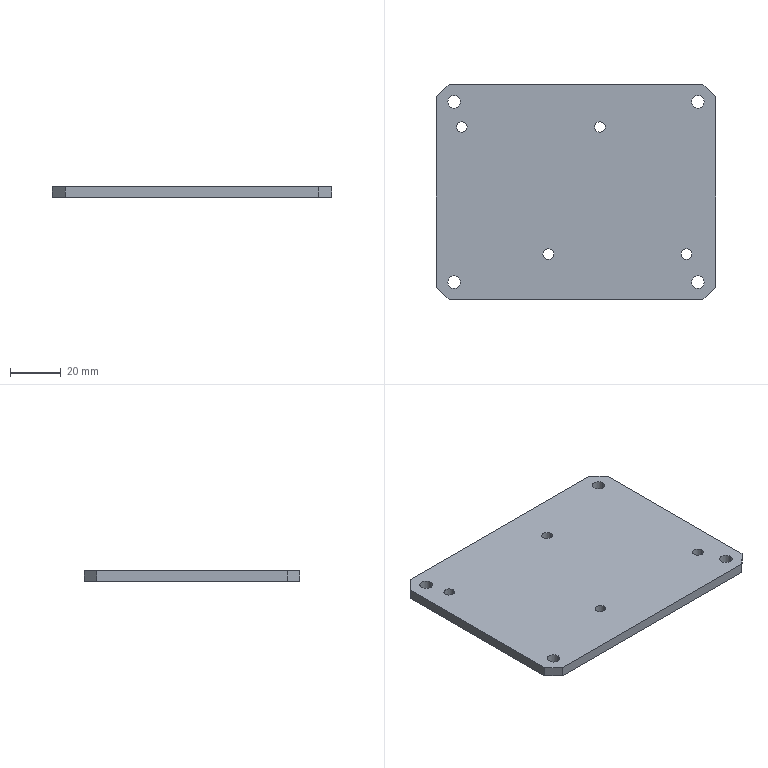Part | SolidWorks | features HoleWzd 2, Chamfer 1, Extrusion 1 | 1 solid | 26 faces | box 110 x 85 x 4 mm | volume 36664 mm3 | cylinder 16 | plane 10 | commonest cylinder face diameters 4.2 x8 5 x8
STEP:
#1=CARTESIAN_POINT('',(-71.534,24.385,4.));
#2=VERTEX_POINT('',#1);
#3=CARTESIAN_POINT('',(-66.534,24.385,4.));
#4=VERTEX_POINT('',#3);
#5=CARTESIAN_POINT('',(-69.034,24.385,4.));
#6=DIRECTION('',(0.,0.,1.));
#7=DIRECTION('',(1.,0.,0.));
#8=AXIS2_PLACEMENT_3D('',#5,#6,#7);
#9=CIRCLE('',#8,2.5);
#10=EDGE_CURVE('',#2,#4,#9,.T.);
#11=ORIENTED_EDGE('',*,*,#10,.T.);
#12=CARTESIAN_POINT('',(-66.534,24.385,0.));
#13=VERTEX_POINT('',#12);
#14=CARTESIAN_POINT('',(-66.534,24.385,0.));
#15=DIRECTION('',(0.,0.,-1.));
#16=VECTOR('',#15,1000.);
#17=LINE('',#14,#16);
#18=EDGE_CURVE('',#4,#13,#17,.T.);
#19=ORIENTED_EDGE('',*,*,#18,.T.);
#20=CARTESIAN_POINT('',(-71.534,24.385,0.));
#21=VERTEX_POINT('',#20);
#22=CARTESIAN_POINT('',(-69.034,24.385,0.));
#23=DIRECTION('',(0.,0.,-1.));
#24=DIRECTION('',(-1.,0.,0.));
#25=AXIS2_PLACEMENT_3D('',#22,#23,#24);
#26=CIRCLE('',#25,2.5);
#27=EDGE_CURVE('',#13,#21,#26,.T.);
#28=ORIENTED_EDGE('',*,*,#27,.T.);
#29=CARTESIAN_POINT('',(-71.534,24.385,0.));
#30=DIRECTION('',(0.,0.,-1.));
#31=VECTOR('',#30,1000.);
#32=LINE('',#29,#31);
#33=EDGE_CURVE('',#2,#21,#32,.T.);
#34=ORIENTED_EDGE('',*,*,#33,.F.);
#35=EDGE_LOOP('',(#11,#19,#28,#34));
#36=FACE_OUTER_BOUND('',#35,.T.);
#37=CARTESIAN_POINT('',(-69.034,24.385,0.));
#38=DIRECTION('',(0.,0.,-1.));
#39=DIRECTION('',(-1.,0.,0.));
#40=AXIS2_PLACEMENT_3D('',#37,#38,#39);
#41=CYLINDRICAL_SURFACE('',#40,2.5);
#42=ADVANCED_FACE('',(#36),#41,.F.);
#43=CARTESIAN_POINT('',(-71.534,-46.615,4.));
#44=VERTEX_POINT('',#43);
#45=CARTESIAN_POINT('',(-66.534,-46.615,4.));
#46=VERTEX_POINT('',#45);
#47=CARTESIAN_POINT('',(-69.034,-46.615,4.));
#48=DIRECTION('',(0.,0.,1.));
#49=DIRECTION('',(1.,0.,0.));
#50=AXIS2_PLACEMENT_3D('',#47,#48,#49);
#51=CIRCLE('',#50,2.5);
#52=EDGE_CURVE('',#44,#46,#51,.T.);
#53=ORIENTED_EDGE('',*,*,#52,.T.);
#54=CARTESIAN_POINT('',(-66.534,-46.615,0.));
#55=VERTEX_POINT('',#54);
#56=CARTESIAN_POINT('',(-66.534,-46.615,0.));
#57=DIRECTION('',(0.,0.,-1.));
#58=VECTOR('',#57,1000.);
#59=LINE('',#56,#58);
#60=EDGE_CURVE('',#46,#55,#59,.T.);
#61=ORIENTED_EDGE('',*,*,#60,.T.);
#62=CARTESIAN_POINT('',(-71.534,-46.615,0.));
#63=VERTEX_POINT('',#62);
#64=CARTESIAN_POINT('',(-69.034,-46.615,0.));
#65=DIRECTION('',(0.,0.,-1.));
#66=DIRECTION('',(-1.,0.,0.));
#67=AXIS2_PLACEMENT_3D('',#64,#65,#66);
#68=CIRCLE('',#67,2.5);
#69=EDGE_CURVE('',#55,#63,#68,.T.);
#70=ORIENTED_EDGE('',*,*,#69,.T.);
#71=CARTESIAN_POINT('',(-71.534,-46.615,0.));
#72=DIRECTION('',(0.,0.,-1.));
#73=VECTOR('',#72,1000.);
#74=LINE('',#71,#73);
#75=EDGE_CURVE('',#44,#63,#74,.T.);
#76=ORIENTED_EDGE('',*,*,#75,.F.);
#77=EDGE_LOOP('',(#53,#61,#70,#76));
#78=FACE_OUTER_BOUND('',#77,.T.);
#79=CARTESIAN_POINT('',(-69.034,-46.615,0.));
#80=DIRECTION('',(0.,0.,-1.));
#81=DIRECTION('',(-1.,0.,0.));
#82=AXIS2_PLACEMENT_3D('',#79,#80,#81);
#83=CYLINDRICAL_SURFACE('',#82,2.5);
#84=ADVANCED_FACE('',(#78),#83,.F.);
#85=CARTESIAN_POINT('',(24.466,-46.615,4.));
#86=VERTEX_POINT('',#85);
#87=CARTESIAN_POINT('',(29.466,-46.615,4.));
#88=VERTEX_POINT('',#87);
#89=CARTESIAN_POINT('',(26.966,-46.615,4.));
#90=DIRECTION('',(0.,0.,1.));
#91=DIRECTION('',(1.,0.,0.));
#92=AXIS2_PLACEMENT_3D('',#89,#90,#91);
#93=CIRCLE('',#92,2.5);
#94=EDGE_CURVE('',#86,#88,#93,.T.);
#95=ORIENTED_EDGE('',*,*,#94,.T.);
#96=CARTESIAN_POINT('',(29.466,-46.615,0.));
#97=VERTEX_POINT('',#96);
#98=CARTESIAN_POINT('',(29.466,-46.615,0.));
#99=DIRECTION('',(0.,0.,-1.));
#100=VECTOR('',#99,1000.);
#101=LINE('',#98,#100);
#102=EDGE_CURVE('',#88,#97,#101,.T.);
#103=ORIENTED_EDGE('',*,*,#102,.T.);
#104=CARTESIAN_POINT('',(24.466,-46.615,0.));
#105=VERTEX_POINT('',#104);
#106=CARTESIAN_POINT('',(26.966,-46.615,0.));
#107=DIRECTION('',(0.,0.,-1.));
#108=DIRECTION('',(-1.,0.,0.));
#109=AXIS2_PLACEMENT_3D('',#106,#107,#108);
#110=CIRCLE('',#109,2.5);
#111=EDGE_CURVE('',#97,#105,#110,.T.);
#112=ORIENTED_EDGE('',*,*,#111,.T.);
#113=CARTESIAN_POINT('',(24.466,-46.615,0.));
#114=DIRECTION('',(0.,0.,-1.));
#115=VECTOR('',#114,1000.);
#116=LINE('',#113,#115);
#117=EDGE_CURVE('',#86,#105,#116,.T.);
#118=ORIENTED_EDGE('',*,*,#117,.F.);
#119=EDGE_LOOP('',(#95,#103,#112,#118));
#120=FACE_OUTER_BOUND('',#119,.T.);
#121=CARTESIAN_POINT('',(26.966,-46.615,0.));
#122=DIRECTION('',(0.,0.,-1.));
#123=DIRECTION('',(-1.,0.,0.));
#124=AXIS2_PLACEMENT_3D('',#121,#122,#123);
#125=CYLINDRICAL_SURFACE('',#124,2.5);
#126=ADVANCED_FACE('',(#120),#125,.F.);
#127=CARTESIAN_POINT('',(24.466,24.385,4.));
#128=VERTEX_POINT('',#127);
#129=CARTESIAN_POINT('',(29.466,24.385,4.));
#130=VERTEX_POINT('',#129);
#131=CARTESIAN_POINT('',(26.966,24.385,4.));
#132=DIRECTION('',(0.,0.,1.));
#133=DIRECTION('',(1.,0.,0.));
#134=AXIS2_PLACEMENT_3D('',#131,#132,#133);
#135=CIRCLE('',#134,2.5);
#136=EDGE_CURVE('',#128,#130,#135,.T.);
#137=ORIENTED_EDGE('',*,*,#136,.T.);
#138=CARTESIAN_POINT('',(29.466,24.385,0.));
#139=VERTEX_POINT('',#138);
#140=CARTESIAN_POINT('',(29.466,24.385,0.));
#141=DIRECTION('',(0.,0.,-1.));
#142=VECTOR('',#141,1000.);
#143=LINE('',#140,#142);
#144=EDGE_CURVE('',#130,#139,#143,.T.);
#145=ORIENTED_EDGE('',*,*,#144,.T.);
#146=CARTESIAN_POINT('',(24.466,24.385,0.));
#147=VERTEX_POINT('',#146);
#148=CARTESIAN_POINT('',(26.966,24.385,0.));
#149=DIRECTION('',(0.,0.,-1.));
#150=DIRECTION('',(-1.,0.,0.));
#151=AXIS2_PLACEMENT_3D('',#148,#149,#150);
#152=CIRCLE('',#151,2.5);
#153=EDGE_CURVE('',#139,#147,#152,.T.);
#154=ORIENTED_EDGE('',*,*,#153,.T.);
#155=CARTESIAN_POINT('',(24.466,24.385,0.));
#156=DIRECTION('',(0.,0.,-1.));
#157=VECTOR('',#156,1000.);
#158=LINE('',#155,#157);
#159=EDGE_CURVE('',#128,#147,#158,.T.);
#160=ORIENTED_EDGE('',*,*,#159,.F.);
#161=EDGE_LOOP('',(#137,#145,#154,#160));
#162=FACE_OUTER_BOUND('',#161,.T.);
#163=CARTESIAN_POINT('',(26.966,24.385,0.));
#164=DIRECTION('',(0.,0.,-1.));
#165=DIRECTION('',(-1.,0.,0.));
#166=AXIS2_PLACEMENT_3D('',#163,#164,#165);
#167=CYLINDRICAL_SURFACE('',#166,2.5);
#168=ADVANCED_FACE('',(#162),#167,.F.);
#169=CARTESIAN_POINT('',(-68.134,14.495,0.));
#170=VERTEX_POINT('',#169);
#171=CARTESIAN_POINT('',(-63.934,14.495,0.));
#172=VERTEX_POINT('',#171);
#173=CARTESIAN_POINT('',(-66.034,14.495,0.));
#174=DIRECTION('',(0.,0.,1.));
#175=DIRECTION('',(1.,0.,0.));
#176=AXIS2_PLACEMENT_3D('',#173,#174,#175);
#177=CIRCLE('',#176,2.1);
#178=EDGE_CURVE('',#170,#172,#177,.T.);
#179=ORIENTED_EDGE('',*,*,#178,.F.);
#180=CARTESIAN_POINT('',(-68.134,14.495,4.));
#181=VERTEX_POINT('',#180);
#182=CARTESIAN_POINT('',(-68.134,14.495,4.));
#183=DIRECTION('',(0.,0.,1.));
#184=VECTOR('',#183,1000.);
#185=LINE('',#182,#184);
#186=EDGE_CURVE('',#170,#181,#185,.T.);
#187=ORIENTED_EDGE('',*,*,#186,.T.);
#188=CARTESIAN_POINT('',(-63.934,14.495,4.));
#189=VERTEX_POINT('',#188);
#190=CARTESIAN_POINT('',(-66.034,14.495,4.));
#191=DIRECTION('',(0.,0.,1.));
#192=DIRECTION('',(1.,0.,0.));
#193=AXIS2_PLACEMENT_3D('',#190,#191,#192);
#194=CIRCLE('',#193,2.1);
#195=EDGE_CURVE('',#181,#189,#194,.T.);
#196=ORIENTED_EDGE('',*,*,#195,.T.);
#197=CARTESIAN_POINT('',(-63.934,14.495,4.));
#198=DIRECTION('',(0.,0.,1.));
#199=VECTOR('',#198,1000.);
#200=LINE('',#197,#199);
#201=EDGE_CURVE('',#172,#189,#200,.T.);
#202=ORIENTED_EDGE('',*,*,#201,.F.);
#203=EDGE_LOOP('',(#179,#187,#196,#202));
#204=FACE_OUTER_BOUND('',#203,.T.);
#205=CARTESIAN_POINT('',(-66.034,14.495,4.));
#206=DIRECTION('',(0.,0.,1.));
#207=DIRECTION('',(1.,0.,0.));
#208=AXIS2_PLACEMENT_3D('',#205,#206,#207);
#209=CYLINDRICAL_SURFACE('',#208,2.1);
#210=ADVANCED_FACE('',(#204),#209,.F.);
#211=CARTESIAN_POINT('',(-34.054,-35.615,0.));
#212=VERTEX_POINT('',#211);
#213=CARTESIAN_POINT('',(-29.854,-35.615,0.));
#214=VERTEX_POINT('',#213);
#215=CARTESIAN_POINT('',(-31.954,-35.615,0.));
#216=DIRECTION('',(0.,0.,1.));
#217=DIRECTION('',(1.,0.,0.));
#218=AXIS2_PLACEMENT_3D('',#215,#216,#217);
#219=CIRCLE('',#218,2.1);
#220=EDGE_CURVE('',#212,#214,#219,.T.);
#221=ORIENTED_EDGE('',*,*,#220,.F.);
#222=CARTESIAN_POINT('',(-34.054,-35.615,4.));
#223=VERTEX_POINT('',#222);
#224=CARTESIAN_POINT('',(-34.054,-35.615,4.));
#225=DIRECTION('',(0.,0.,1.));
#226=VECTOR('',#225,1000.);
#227=LINE('',#224,#226);
#228=EDGE_CURVE('',#212,#223,#227,.T.);
#229=ORIENTED_EDGE('',*,*,#228,.T.);
#230=CARTESIAN_POINT('',(-29.854,-35.615,4.));
#231=VERTEX_POINT('',#230);
#232=CARTESIAN_POINT('',(-31.954,-35.615,4.));
#233=DIRECTION('',(0.,0.,1.));
#234=DIRECTION('',(1.,0.,0.));
#235=AXIS2_PLACEMENT_3D('',#232,#233,#234);
#236=CIRCLE('',#235,2.1);
#237=EDGE_CURVE('',#223,#231,#236,.T.);
#238=ORIENTED_EDGE('',*,*,#237,.T.);
#239=CARTESIAN_POINT('',(-29.854,-35.615,4.));
#240=DIRECTION('',(0.,0.,1.));
#241=VECTOR('',#240,1000.);
#242=LINE('',#239,#241);
#243=EDGE_CURVE('',#214,#231,#242,.T.);
#244=ORIENTED_EDGE('',*,*,#243,.F.);
#245=EDGE_LOOP('',(#221,#229,#238,#244));
#246=FACE_OUTER_BOUND('',#245,.T.);
#247=CARTESIAN_POINT('',(-31.954,-35.615,4.));
#248=DIRECTION('',(0.,0.,1.));
#249=DIRECTION('',(1.,0.,0.));
#250=AXIS2_PLACEMENT_3D('',#247,#248,#249);
#251=CYLINDRICAL_SURFACE('',#250,2.1);
#252=ADVANCED_FACE('',(#246),#251,.F.);
#253=CARTESIAN_POINT('',(-13.714,14.495,0.));
#254=VERTEX_POINT('',#253);
#255=CARTESIAN_POINT('',(-9.514,14.495,0.));
#256=VERTEX_POINT('',#255);
#257=CARTESIAN_POINT('',(-11.614,14.495,0.));
#258=DIRECTION('',(0.,0.,1.));
#259=DIRECTION('',(1.,0.,0.));
#260=AXIS2_PLACEMENT_3D('',#257,#258,#259);
#261=CIRCLE('',#260,2.1);
#262=EDGE_CURVE('',#254,#256,#261,.T.);
#263=ORIENTED_EDGE('',*,*,#262,.F.);
#264=CARTESIAN_POINT('',(-13.714,14.495,4.));
#265=VERTEX_POINT('',#264);
#266=CARTESIAN_POINT('',(-13.714,14.495,4.));
#267=DIRECTION('',(0.,0.,1.));
#268=VECTOR('',#267,1000.);
#269=LINE('',#266,#268);
#270=EDGE_CURVE('',#254,#265,#269,.T.);
#271=ORIENTED_EDGE('',*,*,#270,.T.);
#272=CARTESIAN_POINT('',(-9.514,14.495,4.));
#273=VERTEX_POINT('',#272);
#274=CARTESIAN_POINT('',(-11.614,14.495,4.));
#275=DIRECTION('',(0.,0.,1.));
#276=DIRECTION('',(1.,0.,0.));
#277=AXIS2_PLACEMENT_3D('',#274,#275,#276);
#278=CIRCLE('',#277,2.1);
#279=EDGE_CURVE('',#265,#273,#278,.T.);
#280=ORIENTED_EDGE('',*,*,#279,.T.);
#281=CARTESIAN_POINT('',(-9.514,14.495,4.));
#282=DIRECTION('',(0.,0.,1.));
#283=VECTOR('',#282,1000.);
#284=LINE('',#281,#283);
#285=EDGE_CURVE('',#256,#273,#284,.T.);
#286=ORIENTED_EDGE('',*,*,#285,.F.);
#287=EDGE_LOOP('',(#263,#271,#280,#286));
#288=FACE_OUTER_BOUND('',#287,.T.);
#289=CARTESIAN_POINT('',(-11.614,14.495,4.));
#290=DIRECTION('',(0.,0.,1.));
#291=DIRECTION('',(1.,0.,0.));
#292=AXIS2_PLACEMENT_3D('',#289,#290,#291);
#293=CYLINDRICAL_SURFACE('',#292,2.1);
#294=ADVANCED_FACE('',(#288),#293,.F.);
#295=CARTESIAN_POINT('',(20.366,-35.615,0.));
#296=VERTEX_POINT('',#295);
#297=CARTESIAN_POINT('',(24.566,-35.615,0.));
#298=VERTEX_POINT('',#297);
#299=CARTESIAN_POINT('',(22.466,-35.615,0.));
#300=DIRECTION('',(0.,0.,1.));
#301=DIRECTION('',(1.,0.,0.));
#302=AXIS2_PLACEMENT_3D('',#299,#300,#301);
#303=CIRCLE('',#302,2.1);
#304=EDGE_CURVE('',#296,#298,#303,.T.);
#305=ORIENTED_EDGE('',*,*,#304,.F.);
#306=CARTESIAN_POINT('',(20.366,-35.615,4.));
#307=VERTEX_POINT('',#306);
#308=CARTESIAN_POINT('',(20.366,-35.615,4.));
#309=DIRECTION('',(0.,0.,1.));
#310=VECTOR('',#309,1000.);
#311=LINE('',#308,#310);
#312=EDGE_CURVE('',#296,#307,#311,.T.);
#313=ORIENTED_EDGE('',*,*,#312,.T.);
#314=CARTESIAN_POINT('',(24.566,-35.615,4.));
#315=VERTEX_POINT('',#314);
#316=CARTESIAN_POINT('',(22.466,-35.615,4.));
#317=DIRECTION('',(0.,0.,1.));
#318=DIRECTION('',(1.,0.,0.));
#319=AXIS2_PLACEMENT_3D('',#316,#317,#318);
#320=CIRCLE('',#319,2.1);
#321=EDGE_CURVE('',#307,#315,#320,.T.);
#322=ORIENTED_EDGE('',*,*,#321,.T.);
#323=CARTESIAN_POINT('',(24.566,-35.615,4.));
#324=DIRECTION('',(0.,0.,1.));
#325=VECTOR('',#324,1000.);
#326=LINE('',#323,#325);
#327=EDGE_CURVE('',#298,#315,#326,.T.);
#328=ORIENTED_EDGE('',*,*,#327,.F.);
#329=EDGE_LOOP('',(#305,#313,#322,#328));
#330=FACE_OUTER_BOUND('',#329,.T.);
#331=CARTESIAN_POINT('',(22.466,-35.615,4.));
#332=DIRECTION('',(0.,0.,1.));
#333=DIRECTION('',(1.,0.,0.));
#334=AXIS2_PLACEMENT_3D('',#331,#332,#333);
#335=CYLINDRICAL_SURFACE('',#334,2.1);
#336=ADVANCED_FACE('',(#330),#335,.F.);
#337=CARTESIAN_POINT('',(-69.034,24.385,0.));
#338=DIRECTION('',(0.,0.,-1.));
#339=DIRECTION('',(-1.,0.,0.));
#340=AXIS2_PLACEMENT_3D('',#337,#338,#339);
#341=CIRCLE('',#340,2.5);
#342=EDGE_CURVE('',#21,#13,#341,.T.);
#343=ORIENTED_EDGE('',*,*,#342,.F.);
#344=ORIENTED_EDGE('',*,*,#27,.F.);
#345=EDGE_LOOP('',(#343,#344));
#346=FACE_BOUND('',#345,.T.);
#347=CARTESIAN_POINT('',(-69.034,-46.615,0.));
#348=DIRECTION('',(0.,0.,-1.));
#349=DIRECTION('',(-1.,0.,0.));
#350=AXIS2_PLACEMENT_3D('',#347,#348,#349);
#351=CIRCLE('',#350,2.5);
#352=EDGE_CURVE('',#63,#55,#351,.T.);
#353=ORIENTED_EDGE('',*,*,#352,.F.);
#354=ORIENTED_EDGE('',*,*,#69,.F.);
#355=EDGE_LOOP('',(#353,#354));
#356=FACE_BOUND('',#355,.T.);
#357=CARTESIAN_POINT('',(26.966,-46.615,0.));
#358=DIRECTION('',(0.,0.,-1.));
#359=DIRECTION('',(-1.,0.,0.));
#360=AXIS2_PLACEMENT_3D('',#357,#358,#359);
#361=CIRCLE('',#360,2.5);
#362=EDGE_CURVE('',#105,#97,#361,.T.);
#363=ORIENTED_EDGE('',*,*,#362,.F.);
#364=ORIENTED_EDGE('',*,*,#111,.F.);
#365=EDGE_LOOP('',(#363,#364));
#366=FACE_BOUND('',#365,.T.);
#367=CARTESIAN_POINT('',(-71.034,-53.615,0.));
#368=VERTEX_POINT('',#367);
#369=CARTESIAN_POINT('',(28.966,-53.615,0.));
#370=VERTEX_POINT('',#369);
#371=CARTESIAN_POINT('',(-76.034,-53.615,0.));
#372=DIRECTION('',(1.,0.,0.));
#373=VECTOR('',#372,1000.);
#374=LINE('',#371,#373);
#375=EDGE_CURVE('',#368,#370,#374,.T.);
#376=ORIENTED_EDGE('',*,*,#375,.F.);
#377=CARTESIAN_POINT('',(-76.034,-48.615,0.));
#378=VERTEX_POINT('',#377);
#379=CARTESIAN_POINT('',(-71.034,-53.615,0.));
#380=DIRECTION('',(-0.7071,0.7071,0.));
#381=VECTOR('',#380,1000.);
#382=LINE('',#379,#381);
#383=EDGE_CURVE('',#368,#378,#382,.T.);
#384=ORIENTED_EDGE('',*,*,#383,.T.);
#385=CARTESIAN_POINT('',(-76.034,26.385,0.));
#386=VERTEX_POINT('',#385);
#387=CARTESIAN_POINT('',(-76.034,31.385,0.));
#388=DIRECTION('',(0.,-1.,0.));
#389=VECTOR('',#388,1000.);
#390=LINE('',#387,#389);
#391=EDGE_CURVE('',#386,#378,#390,.T.);
#392=ORIENTED_EDGE('',*,*,#391,.F.);
#393=CARTESIAN_POINT('',(-71.034,31.385,0.));
#394=VERTEX_POINT('',#393);
#395=CARTESIAN_POINT('',(-76.034,26.385,0.));
#396=DIRECTION('',(0.7071,0.7071,0.));
#397=VECTOR('',#396,1000.);
#398=LINE('',#395,#397);
#399=EDGE_CURVE('',#386,#394,#398,.T.);
#400=ORIENTED_EDGE('',*,*,#399,.T.);
#401=CARTESIAN_POINT('',(28.966,31.385,0.));
#402=VERTEX_POINT('',#401);
#403=CARTESIAN_POINT('',(-76.034,31.385,0.));
#404=DIRECTION('',(-1.,0.,0.));
#405=VECTOR('',#404,1000.);
#406=LINE('',#403,#405);
#407=EDGE_CURVE('',#402,#394,#406,.T.);
#408=ORIENTED_EDGE('',*,*,#407,.F.);
#409=CARTESIAN_POINT('',(33.966,26.385,0.));
#410=VERTEX_POINT('',#409);
#411=CARTESIAN_POINT('',(28.966,31.385,0.));
#412=DIRECTION('',(0.7071,-0.7071,0.));
#413=VECTOR('',#412,1000.);
#414=LINE('',#411,#413);
#415=EDGE_CURVE('',#402,#410,#414,.T.);
#416=ORIENTED_EDGE('',*,*,#415,.T.);
#417=CARTESIAN_POINT('',(33.966,-48.615,0.));
#418=VERTEX_POINT('',#417);
#419=CARTESIAN_POINT('',(33.966,31.385,0.));
#420=DIRECTION('',(0.,1.,0.));
#421=VECTOR('',#420,1000.);
#422=LINE('',#419,#421);
#423=EDGE_CURVE('',#418,#410,#422,.T.);
#424=ORIENTED_EDGE('',*,*,#423,.F.);
#425=CARTESIAN_POINT('',(33.966,-48.615,0.));
#426=DIRECTION('',(-0.7071,-0.7071,0.));
#427=VECTOR('',#426,1000.);
#428=LINE('',#425,#427);
#429=EDGE_CURVE('',#418,#370,#428,.T.);
#430=ORIENTED_EDGE('',*,*,#429,.T.);
#431=EDGE_LOOP('',(#376,#384,#392,#400,#408,#416,#424,#430));
#432=FACE_OUTER_BOUND('',#431,.T.);
#433=CARTESIAN_POINT('',(22.466,-35.615,0.));
#434=DIRECTION('',(0.,0.,1.));
#435=DIRECTION('',(1.,0.,0.));
#436=AXIS2_PLACEMENT_3D('',#433,#434,#435);
#437=CIRCLE('',#436,2.1);
#438=EDGE_CURVE('',#298,#296,#437,.T.);
#439=ORIENTED_EDGE('',*,*,#438,.T.);
#440=ORIENTED_EDGE('',*,*,#304,.T.);
#441=EDGE_LOOP('',(#439,#440));
#442=FACE_BOUND('',#441,.T.);
#443=CARTESIAN_POINT('',(-11.614,14.495,0.));
#444=DIRECTION('',(0.,0.,1.));
#445=DIRECTION('',(1.,0.,0.));
#446=AXIS2_PLACEMENT_3D('',#443,#444,#445);
#447=CIRCLE('',#446,2.1);
#448=EDGE_CURVE('',#256,#254,#447,.T.);
#449=ORIENTED_EDGE('',*,*,#448,.T.);
#450=ORIENTED_EDGE('',*,*,#262,.T.);
#451=EDGE_LOOP('',(#449,#450));
#452=FACE_BOUND('',#451,.T.);
#453=CARTESIAN_POINT('',(-31.954,-35.615,0.));
#454=DIRECTION('',(0.,0.,1.));
#455=DIRECTION('',(1.,0.,0.));
#456=AXIS2_PLACEMENT_3D('',#453,#454,#455);
#457=CIRCLE('',#456,2.1);
#458=EDGE_CURVE('',#214,#212,#457,.T.);
#459=ORIENTED_EDGE('',*,*,#458,.T.);
#460=ORIENTED_EDGE('',*,*,#220,.T.);
#461=EDGE_LOOP('',(#459,#460));
#462=FACE_BOUND('',#461,.T.);
#463=CARTESIAN_POINT('',(-66.034,14.495,0.));
#464=DIRECTION('',(0.,0.,1.));
#465=DIRECTION('',(1.,0.,0.));
#466=AXIS2_PLACEMENT_3D('',#463,#464,#465);
#467=CIRCLE('',#466,2.1);
#468=EDGE_CURVE('',#172,#170,#467,.T.);
#469=ORIENTED_EDGE('',*,*,#468,.T.);
#470=ORIENTED_EDGE('',*,*,#178,.T.);
#471=EDGE_LOOP('',(#469,#470));
#472=FACE_BOUND('',#471,.T.);
#473=CARTESIAN_POINT('',(26.966,24.385,0.));
#474=DIRECTION('',(0.,0.,-1.));
#475=DIRECTION('',(-1.,0.,0.));
#476=AXIS2_PLACEMENT_3D('',#473,#474,#475);
#477=CIRCLE('',#476,2.5);
#478=EDGE_CURVE('',#147,#139,#477,.T.);
#479=ORIENTED_EDGE('',*,*,#478,.F.);
#480=ORIENTED_EDGE('',*,*,#153,.F.);
#481=EDGE_LOOP('',(#479,#480));
#482=FACE_BOUND('',#481,.T.);
#483=CARTESIAN_POINT('',(0.,0.,0.));
#484=DIRECTION('',(0.,0.,1.));
#485=DIRECTION('',(1.,0.,0.));
#486=AXIS2_PLACEMENT_3D('',#483,#484,#485);
#487=PLANE('',#486);
#488=ADVANCED_FACE('',(#346,#356,#366,#432,#442,#452,#462,#472,#482),#487,.F.);
#489=ORIENTED_EDGE('',*,*,#391,.T.);
#490=CARTESIAN_POINT('',(-76.034,-48.615,4.));
#491=VERTEX_POINT('',#490);
#492=CARTESIAN_POINT('',(-76.034,-48.615,4.));
#493=DIRECTION('',(0.,0.,1.));
#494=VECTOR('',#493,1000.);
#495=LINE('',#492,#494);
#496=EDGE_CURVE('',#378,#491,#495,.T.);
#497=ORIENTED_EDGE('',*,*,#496,.T.);
#498=CARTESIAN_POINT('',(-76.034,26.385,4.));
#499=VERTEX_POINT('',#498);
#500=CARTESIAN_POINT('',(-76.034,31.385,4.));
#501=DIRECTION('',(0.,-1.,0.));
#502=VECTOR('',#501,1000.);
#503=LINE('',#500,#502);
#504=EDGE_CURVE('',#499,#491,#503,.T.);
#505=ORIENTED_EDGE('',*,*,#504,.F.);
#506=CARTESIAN_POINT('',(-76.034,26.385,4.));
#507=DIRECTION('',(0.,0.,-1.));
#508=VECTOR('',#507,1000.);
#509=LINE('',#506,#508);
#510=EDGE_CURVE('',#499,#386,#509,.T.);
#511=ORIENTED_EDGE('',*,*,#510,.T.);
#512=EDGE_LOOP('',(#489,#497,#505,#511));
#513=FACE_OUTER_BOUND('',#512,.T.);
#514=CARTESIAN_POINT('',(-76.034,31.385,4.));
#515=DIRECTION('',(1.,0.,0.));
#516=DIRECTION('',(0.,0.,-1.));
#517=AXIS2_PLACEMENT_3D('',#514,#515,#516);
#518=PLANE('',#517);
#519=ADVANCED_FACE('',(#513),#518,.F.);
#520=CARTESIAN_POINT('',(-71.034,-53.615,4.));
#521=VERTEX_POINT('',#520);
#522=CARTESIAN_POINT('',(28.966,-53.615,4.));
#523=VERTEX_POINT('',#522);
#524=CARTESIAN_POINT('',(-76.034,-53.615,4.));
#525=DIRECTION('',(1.,0.,0.));
#526=VECTOR('',#525,1000.);
#527=LINE('',#524,#526);
#528=EDGE_CURVE('',#521,#523,#527,.T.);
#529=ORIENTED_EDGE('',*,*,#528,.F.);
#530=CARTESIAN_POINT('',(-71.034,-53.615,4.));
#531=DIRECTION('',(0.,0.,-1.));
#532=VECTOR('',#531,1000.);
#533=LINE('',#530,#532);
#534=EDGE_CURVE('',#521,#368,#533,.T.);
#535=ORIENTED_EDGE('',*,*,#534,.T.);
#536=ORIENTED_EDGE('',*,*,#375,.T.);
#537=CARTESIAN_POINT('',(28.966,-53.615,4.));
#538=DIRECTION('',(0.,0.,1.));
#539=VECTOR('',#538,1000.);
#540=LINE('',#537,#539);
#541=EDGE_CURVE('',#370,#523,#540,.T.);
#542=ORIENTED_EDGE('',*,*,#541,.T.);
#543=EDGE_LOOP('',(#529,#535,#536,#542));
#544=FACE_OUTER_BOUND('',#543,.T.);
#545=CARTESIAN_POINT('',(-76.034,-53.615,4.));
#546=DIRECTION('',(0.,1.,0.));
#547=DIRECTION('',(0.,0.,1.));
#548=AXIS2_PLACEMENT_3D('',#545,#546,#547);
#549=PLANE('',#548);
#550=ADVANCED_FACE('',(#544),#549,.F.);
#551=CARTESIAN_POINT('',(33.966,-48.615,4.));
#552=VERTEX_POINT('',#551);
#553=CARTESIAN_POINT('',(33.966,26.385,4.));
#554=VERTEX_POINT('',#553);
#555=CARTESIAN_POINT('',(33.966,31.385,4.));
#556=DIRECTION('',(0.,1.,0.));
#557=VECTOR('',#556,1000.);
#558=LINE('',#555,#557);
#559=EDGE_CURVE('',#552,#554,#558,.T.);
#560=ORIENTED_EDGE('',*,*,#559,.F.);
#561=CARTESIAN_POINT('',(33.966,-48.615,4.));
#562=DIRECTION('',(0.,0.,-1.));
#563=VECTOR('',#562,1000.);
#564=LINE('',#561,#563);
#565=EDGE_CURVE('',#552,#418,#564,.T.);
#566=ORIENTED_EDGE('',*,*,#565,.T.);
#567=ORIENTED_EDGE('',*,*,#423,.T.);
#568=CARTESIAN_POINT('',(33.966,26.385,4.));
#569=DIRECTION('',(0.,0.,1.));
#570=VECTOR('',#569,1000.);
#571=LINE('',#568,#570);
#572=EDGE_CURVE('',#410,#554,#571,.T.);
#573=ORIENTED_EDGE('',*,*,#572,.T.);
#574=EDGE_LOOP('',(#560,#566,#567,#573));
#575=FACE_OUTER_BOUND('',#574,.T.);
#576=CARTESIAN_POINT('',(33.966,31.385,4.));
#577=DIRECTION('',(-1.,0.,0.));
#578=DIRECTION('',(0.,-1.,0.));
#579=AXIS2_PLACEMENT_3D('',#576,#577,#578);
#580=PLANE('',#579);
#581=ADVANCED_FACE('',(#575),#580,.F.);
#582=ORIENTED_EDGE('',*,*,#407,.T.);
#583=CARTESIAN_POINT('',(-71.034,31.385,4.));
#584=VERTEX_POINT('',#583);
#585=CARTESIAN_POINT('',(-71.034,31.385,4.));
#586=DIRECTION('',(0.,0.,1.));
#587=VECTOR('',#586,1000.);
#588=LINE('',#585,#587);
#589=EDGE_CURVE('',#394,#584,#588,.T.);
#590=ORIENTED_EDGE('',*,*,#589,.T.);
#591=CARTESIAN_POINT('',(28.966,31.385,4.));
#592=VERTEX_POINT('',#591);
#593=CARTESIAN_POINT('',(-76.034,31.385,4.));
#594=DIRECTION('',(-1.,0.,0.));
#595=VECTOR('',#594,1000.);
#596=LINE('',#593,#595);
#597=EDGE_CURVE('',#592,#584,#596,.T.);
#598=ORIENTED_EDGE('',*,*,#597,.F.);
#599=CARTESIAN_POINT('',(28.966,31.385,4.));
#600=DIRECTION('',(0.,0.,-1.));
#601=VECTOR('',#600,1000.);
#602=LINE('',#599,#601);
#603=EDGE_CURVE('',#592,#402,#602,.T.);
#604=ORIENTED_EDGE('',*,*,#603,.T.);
#605=EDGE_LOOP('',(#582,#590,#598,#604));
#606=FACE_OUTER_BOUND('',#605,.T.);
#607=CARTESIAN_POINT('',(-76.034,31.385,4.));
#608=DIRECTION('',(0.,-1.,0.));
#609=DIRECTION('',(0.,0.,-1.));
#610=AXIS2_PLACEMENT_3D('',#607,#608,#609);
#611=PLANE('',#610);
#612=ADVANCED_FACE('',(#606),#611,.F.);
#613=ORIENTED_EDGE('',*,*,#10,.F.);
#614=CARTESIAN_POINT('',(-69.034,24.385,4.));
#615=DIRECTION('',(0.,0.,1.));
#616=DIRECTION('',(1.,0.,0.));
#617=AXIS2_PLACEMENT_3D('',#614,#615,#616);
#618=CIRCLE('',#617,2.5);
#619=EDGE_CURVE('',#4,#2,#618,.T.);
#620=ORIENTED_EDGE('',*,*,#619,.F.);
#621=EDGE_LOOP('',(#613,#620));
#622=FACE_BOUND('',#621,.T.);
#623=ORIENTED_EDGE('',*,*,#52,.F.);
#624=CARTESIAN_POINT('',(-69.034,-46.615,4.));
#625=DIRECTION('',(0.,0.,1.));
#626=DIRECTION('',(1.,0.,0.));
#627=AXIS2_PLACEMENT_3D('',#624,#625,#626);
#628=CIRCLE('',#627,2.5);
#629=EDGE_CURVE('',#46,#44,#628,.T.);
#630=ORIENTED_EDGE('',*,*,#629,.F.);
#631=EDGE_LOOP('',(#623,#630));
#632=FACE_BOUND('',#631,.T.);
#633=ORIENTED_EDGE('',*,*,#94,.F.);
#634=CARTESIAN_POINT('',(26.966,-46.615,4.));
#635=DIRECTION('',(0.,0.,1.));
#636=DIRECTION('',(1.,0.,0.));
#637=AXIS2_PLACEMENT_3D('',#634,#635,#636);
#638=CIRCLE('',#637,2.5);
#639=EDGE_CURVE('',#88,#86,#638,.T.);
#640=ORIENTED_EDGE('',*,*,#639,.F.);
#641=EDGE_LOOP('',(#633,#640));
#642=FACE_BOUND('',#641,.T.);
#643=ORIENTED_EDGE('',*,*,#136,.F.);
#644=CARTESIAN_POINT('',(26.966,24.385,4.));
#645=DIRECTION('',(0.,0.,1.));
#646=DIRECTION('',(1.,0.,0.));
#647=AXIS2_PLACEMENT_3D('',#644,#645,#646);
#648=CIRCLE('',#647,2.5);
#649=EDGE_CURVE('',#130,#128,#648,.T.);
#650=ORIENTED_EDGE('',*,*,#649,.F.);
#651=EDGE_LOOP('',(#643,#650));
#652=FACE_BOUND('',#651,.T.);
#653=CARTESIAN_POINT('',(-66.034,14.495,4.));
#654=DIRECTION('',(0.,0.,1.));
#655=DIRECTION('',(1.,0.,0.));
#656=AXIS2_PLACEMENT_3D('',#653,#654,#655);
#657=CIRCLE('',#656,2.1);
#658=EDGE_CURVE('',#189,#181,#657,.T.);
#659=ORIENTED_EDGE('',*,*,#658,.F.);
#660=ORIENTED_EDGE('',*,*,#195,.F.);
#661=EDGE_LOOP('',(#659,#660));
#662=FACE_BOUND('',#661,.T.);
#663=CARTESIAN_POINT('',(-31.954,-35.615,4.));
#664=DIRECTION('',(0.,0.,1.));
#665=DIRECTION('',(1.,0.,0.));
#666=AXIS2_PLACEMENT_3D('',#663,#664,#665);
#667=CIRCLE('',#666,2.1);
#668=EDGE_CURVE('',#231,#223,#667,.T.);
#669=ORIENTED_EDGE('',*,*,#668,.F.);
#670=ORIENTED_EDGE('',*,*,#237,.F.);
#671=EDGE_LOOP('',(#669,#670));
#672=FACE_BOUND('',#671,.T.);
#673=CARTESIAN_POINT('',(-11.614,14.495,4.));
#674=DIRECTION('',(0.,0.,1.));
#675=DIRECTION('',(1.,0.,0.));
#676=AXIS2_PLACEMENT_3D('',#673,#674,#675);
#677=CIRCLE('',#676,2.1);
#678=EDGE_CURVE('',#273,#265,#677,.T.);
#679=ORIENTED_EDGE('',*,*,#678,.F.);
#680=ORIENTED_EDGE('',*,*,#279,.F.);
#681=EDGE_LOOP('',(#679,#680));
#682=FACE_BOUND('',#681,.T.);
#683=CARTESIAN_POINT('',(22.466,-35.615,4.));
#684=DIRECTION('',(0.,0.,1.));
#685=DIRECTION('',(1.,0.,0.));
#686=AXIS2_PLACEMENT_3D('',#683,#684,#685);
#687=CIRCLE('',#686,2.1);
#688=EDGE_CURVE('',#315,#307,#687,.T.);
#689=ORIENTED_EDGE('',*,*,#688,.F.);
#690=ORIENTED_EDGE('',*,*,#321,.F.);
#691=EDGE_LOOP('',(#689,#690));
#692=FACE_BOUND('',#691,.T.);
#693=ORIENTED_EDGE('',*,*,#504,.T.);
#694=CARTESIAN_POINT('',(-62.324,-62.324,4.));
#695=DIRECTION('',(0.7071,-0.7071,0.));
#696=VECTOR('',#695,1000.);
#697=LINE('',#694,#696);
#698=EDGE_CURVE('',#491,#521,#697,.T.);
#699=ORIENTED_EDGE('',*,*,#698,.T.);
#700=ORIENTED_EDGE('',*,*,#528,.T.);
#701=CARTESIAN_POINT('',(41.291,-41.291,4.));
#702=DIRECTION('',(0.7071,0.7071,0.));
#703=VECTOR('',#702,1000.);
#704=LINE('',#701,#703);
#705=EDGE_CURVE('',#523,#552,#704,.T.);
#706=ORIENTED_EDGE('',*,*,#705,.T.);
#707=ORIENTED_EDGE('',*,*,#559,.T.);
#708=CARTESIAN_POINT('',(30.176,30.176,4.));
#709=DIRECTION('',(-0.7071,0.7071,0.));
#710=VECTOR('',#709,1000.);
#711=LINE('',#708,#710);
#712=EDGE_CURVE('',#554,#592,#711,.T.);
#713=ORIENTED_EDGE('',*,*,#712,.T.);
#714=ORIENTED_EDGE('',*,*,#597,.T.);
#715=CARTESIAN_POINT('',(-51.209,51.209,4.));
#716=DIRECTION('',(-0.7071,-0.7071,0.));
#717=VECTOR('',#716,1000.);
#718=LINE('',#715,#717);
#719=EDGE_CURVE('',#584,#499,#718,.T.);
#720=ORIENTED_EDGE('',*,*,#719,.T.);
#721=EDGE_LOOP('',(#693,#699,#700,#706,#707,#713,#714,#720));
#722=FACE_OUTER_BOUND('',#721,.T.);
#723=CARTESIAN_POINT('',(0.,0.,4.));
#724=DIRECTION('',(0.,0.,1.));
#725=DIRECTION('',(1.,0.,0.));
#726=AXIS2_PLACEMENT_3D('',#723,#724,#725);
#727=PLANE('',#726);
#728=ADVANCED_FACE('',(#622,#632,#642,#652,#662,#672,#682,#692,#722),#727,.T.);
#729=ORIENTED_EDGE('',*,*,#312,.F.);
#730=ORIENTED_EDGE('',*,*,#438,.F.);
#731=ORIENTED_EDGE('',*,*,#327,.T.);
#732=ORIENTED_EDGE('',*,*,#688,.T.);
#733=EDGE_LOOP('',(#729,#730,#731,#732));
#734=FACE_OUTER_BOUND('',#733,.T.);
#735=CARTESIAN_POINT('',(22.466,-35.615,4.));
#736=DIRECTION('',(0.,0.,1.));
#737=DIRECTION('',(1.,0.,0.));
#738=AXIS2_PLACEMENT_3D('',#735,#736,#737);
#739=CYLINDRICAL_SURFACE('',#738,2.1);
#740=ADVANCED_FACE('',(#734),#739,.F.);
#741=ORIENTED_EDGE('',*,*,#270,.F.);
#742=ORIENTED_EDGE('',*,*,#448,.F.);
#743=ORIENTED_EDGE('',*,*,#285,.T.);
#744=ORIENTED_EDGE('',*,*,#678,.T.);
#745=EDGE_LOOP('',(#741,#742,#743,#744));
#746=FACE_OUTER_BOUND('',#745,.T.);
#747=CARTESIAN_POINT('',(-11.614,14.495,4.));
#748=DIRECTION('',(0.,0.,1.));
#749=DIRECTION('',(1.,0.,0.));
#750=AXIS2_PLACEMENT_3D('',#747,#748,#749);
#751=CYLINDRICAL_SURFACE('',#750,2.1);
#752=ADVANCED_FACE('',(#746),#751,.F.);
#753=ORIENTED_EDGE('',*,*,#228,.F.);
#754=ORIENTED_EDGE('',*,*,#458,.F.);
#755=ORIENTED_EDGE('',*,*,#243,.T.);
#756=ORIENTED_EDGE('',*,*,#668,.T.);
#757=EDGE_LOOP('',(#753,#754,#755,#756));
#758=FACE_OUTER_BOUND('',#757,.T.);
#759=CARTESIAN_POINT('',(-31.954,-35.615,4.));
#760=DIRECTION('',(0.,0.,1.));
#761=DIRECTION('',(1.,0.,0.));
#762=AXIS2_PLACEMENT_3D('',#759,#760,#761);
#763=CYLINDRICAL_SURFACE('',#762,2.1);
#764=ADVANCED_FACE('',(#758),#763,.F.);
#765=ORIENTED_EDGE('',*,*,#186,.F.);
#766=ORIENTED_EDGE('',*,*,#468,.F.);
#767=ORIENTED_EDGE('',*,*,#201,.T.);
#768=ORIENTED_EDGE('',*,*,#658,.T.);
#769=EDGE_LOOP('',(#765,#766,#767,#768));
#770=FACE_OUTER_BOUND('',#769,.T.);
#771=CARTESIAN_POINT('',(-66.034,14.495,4.));
#772=DIRECTION('',(0.,0.,1.));
#773=DIRECTION('',(1.,0.,0.));
#774=AXIS2_PLACEMENT_3D('',#771,#772,#773);
#775=CYLINDRICAL_SURFACE('',#774,2.1);
#776=ADVANCED_FACE('',(#770),#775,.F.);
#777=ORIENTED_EDGE('',*,*,#698,.F.);
#778=ORIENTED_EDGE('',*,*,#496,.F.);
#779=ORIENTED_EDGE('',*,*,#383,.F.);
#780=ORIENTED_EDGE('',*,*,#534,.F.);
#781=EDGE_LOOP('',(#777,#778,#779,#780));
#782=FACE_OUTER_BOUND('',#781,.T.);
#783=CARTESIAN_POINT('',(-71.034,-53.615,4.));
#784=DIRECTION('',(0.7071,0.7071,0.));
#785=DIRECTION('',(0.,0.,-1.));
#786=AXIS2_PLACEMENT_3D('',#783,#784,#785);
#787=PLANE('',#786);
#788=ADVANCED_FACE('',(#782),#787,.F.);
#789=ORIENTED_EDGE('',*,*,#719,.F.);
#790=ORIENTED_EDGE('',*,*,#589,.F.);
#791=ORIENTED_EDGE('',*,*,#399,.F.);
#792=ORIENTED_EDGE('',*,*,#510,.F.);
#793=EDGE_LOOP('',(#789,#790,#791,#792));
#794=FACE_OUTER_BOUND('',#793,.T.);
#795=CARTESIAN_POINT('',(-76.034,26.385,4.));
#796=DIRECTION('',(0.7071,-0.7071,0.));
#797=DIRECTION('',(0.,0.,-1.));
#798=AXIS2_PLACEMENT_3D('',#795,#796,#797);
#799=PLANE('',#798);
#800=ADVANCED_FACE('',(#794),#799,.F.);
#801=ORIENTED_EDGE('',*,*,#705,.F.);
#802=ORIENTED_EDGE('',*,*,#541,.F.);
#803=ORIENTED_EDGE('',*,*,#429,.F.);
#804=ORIENTED_EDGE('',*,*,#565,.F.);
#805=EDGE_LOOP('',(#801,#802,#803,#804));
#806=FACE_OUTER_BOUND('',#805,.T.);
#807=CARTESIAN_POINT('',(33.966,-48.615,4.));
#808=DIRECTION('',(-0.7071,0.7071,0.));
#809=DIRECTION('',(0.,0.,-1.));
#810=AXIS2_PLACEMENT_3D('',#807,#808,#809);
#811=PLANE('',#810);
#812=ADVANCED_FACE('',(#806),#811,.F.);
#813=ORIENTED_EDGE('',*,*,#712,.F.);
#814=ORIENTED_EDGE('',*,*,#572,.F.);
#815=ORIENTED_EDGE('',*,*,#415,.F.);
#816=ORIENTED_EDGE('',*,*,#603,.F.);
#817=EDGE_LOOP('',(#813,#814,#815,#816));
#818=FACE_OUTER_BOUND('',#817,.T.);
#819=CARTESIAN_POINT('',(28.966,31.385,4.));
#820=DIRECTION('',(-0.7071,-0.7071,0.));
#821=DIRECTION('',(0.,0.,-1.));
#822=AXIS2_PLACEMENT_3D('',#819,#820,#821);
#823=PLANE('',#822);
#824=ADVANCED_FACE('',(#818),#823,.F.);
#825=ORIENTED_EDGE('',*,*,#144,.F.);
#826=ORIENTED_EDGE('',*,*,#649,.T.);
#827=ORIENTED_EDGE('',*,*,#159,.T.);
#828=ORIENTED_EDGE('',*,*,#478,.T.);
#829=EDGE_LOOP('',(#825,#826,#827,#828));
#830=FACE_OUTER_BOUND('',#829,.T.);
#831=CARTESIAN_POINT('',(26.966,24.385,0.));
#832=DIRECTION('',(0.,0.,-1.));
#833=DIRECTION('',(-1.,0.,0.));
#834=AXIS2_PLACEMENT_3D('',#831,#832,#833);
#835=CYLINDRICAL_SURFACE('',#834,2.5);
#836=ADVANCED_FACE('',(#830),#835,.F.);
#837=ORIENTED_EDGE('',*,*,#102,.F.);
#838=ORIENTED_EDGE('',*,*,#639,.T.);
#839=ORIENTED_EDGE('',*,*,#117,.T.);
#840=ORIENTED_EDGE('',*,*,#362,.T.);
#841=EDGE_LOOP('',(#837,#838,#839,#840));
#842=FACE_OUTER_BOUND('',#841,.T.);
#843=CARTESIAN_POINT('',(26.966,-46.615,0.));
#844=DIRECTION('',(0.,0.,-1.));
#845=DIRECTION('',(-1.,0.,0.));
#846=AXIS2_PLACEMENT_3D('',#843,#844,#845);
#847=CYLINDRICAL_SURFACE('',#846,2.5);
#848=ADVANCED_FACE('',(#842),#847,.F.);
#849=ORIENTED_EDGE('',*,*,#60,.F.);
#850=ORIENTED_EDGE('',*,*,#629,.T.);
#851=ORIENTED_EDGE('',*,*,#75,.T.);
#852=ORIENTED_EDGE('',*,*,#352,.T.);
#853=EDGE_LOOP('',(#849,#850,#851,#852));
#854=FACE_OUTER_BOUND('',#853,.T.);
#855=CARTESIAN_POINT('',(-69.034,-46.615,0.));
#856=DIRECTION('',(0.,0.,-1.));
#857=DIRECTION('',(-1.,0.,0.));
#858=AXIS2_PLACEMENT_3D('',#855,#856,#857);
#859=CYLINDRICAL_SURFACE('',#858,2.5);
#860=ADVANCED_FACE('',(#854),#859,.F.);
#861=ORIENTED_EDGE('',*,*,#18,.F.);
#862=ORIENTED_EDGE('',*,*,#619,.T.);
#863=ORIENTED_EDGE('',*,*,#33,.T.);
#864=ORIENTED_EDGE('',*,*,#342,.T.);
#865=EDGE_LOOP('',(#861,#862,#863,#864));
#866=FACE_OUTER_BOUND('',#865,.T.);
#867=CARTESIAN_POINT('',(-69.034,24.385,0.));
#868=DIRECTION('',(0.,0.,-1.));
#869=DIRECTION('',(-1.,0.,0.));
#870=AXIS2_PLACEMENT_3D('',#867,#868,#869);
#871=CYLINDRICAL_SURFACE('',#870,2.5);
#872=ADVANCED_FACE('',(#866),#871,.F.);
#873=CLOSED_SHELL('',(#42,#84,#126,#168,#210,#252,#294,#336,#488,#519,#550,#581,#612,#728,#740,#752,#764,#776,#788,#800,#812,#824,#836,#848,#860,#872));
#874=MANIFOLD_SOLID_BREP('',#873);
#875=CARTESIAN_POINT('',(0.,0.,0.));
#876=DIRECTION('',(0.,0.,1.));
#877=DIRECTION('',(1.,0.,0.));
#878=AXIS2_PLACEMENT_3D('',#875,#876,#877);
#879=(LENGTH_UNIT()NAMED_UNIT(*)SI_UNIT(.MILLI.,.METRE.));
#880=UNCERTAINTY_MEASURE_WITH_UNIT(LENGTH_MEASURE(0.00001),#879,'','');
#881=(NAMED_UNIT(*)PLANE_ANGLE_UNIT()SI_UNIT($,.RADIAN.));
#882=(NAMED_UNIT(*)SI_UNIT($,.STERADIAN.)SOLID_ANGLE_UNIT());
#883=(GEOMETRIC_REPRESENTATION_CONTEXT(3)GLOBAL_UNCERTAINTY_ASSIGNED_CONTEXT((#880))GLOBAL_UNIT_ASSIGNED_CONTEXT((#879,#881,#882))REPRESENTATION_CONTEXT('',''));
#884=ADVANCED_BREP_SHAPE_REPRESENTATION('',(#874,#878),#883);